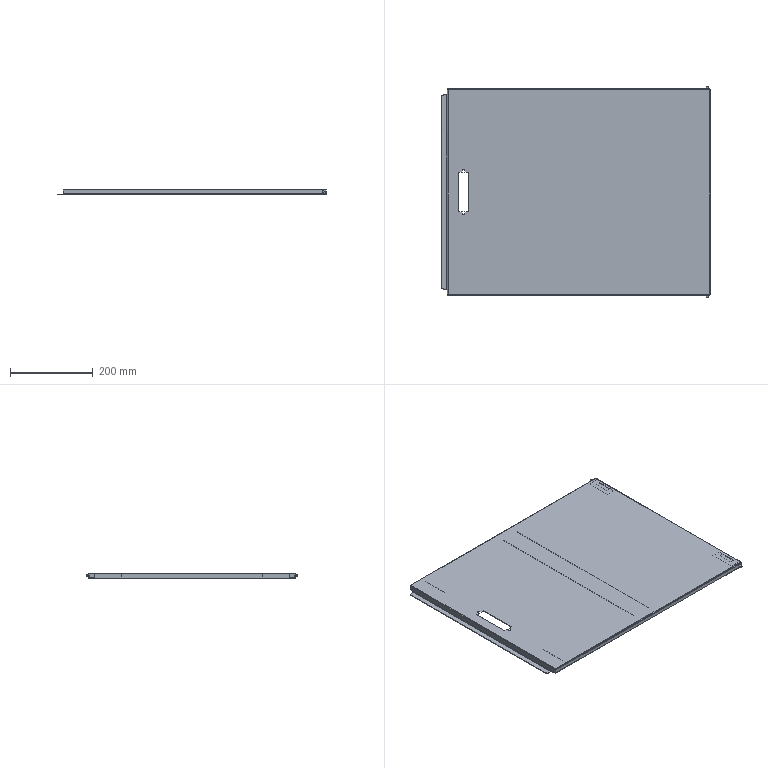Part | SolidWorks | features BaseBody 6 | 6 solids | 198 faces | box 651.5 x 513 x 14.5 mm | volume 623837 mm3 | plane 106 | cylinder 60 | spline 28 | torus 4 | commonest cylinder face diameters 5 x16 1.473 x14 4.473 x14 9 x12 6 x2 10 x2